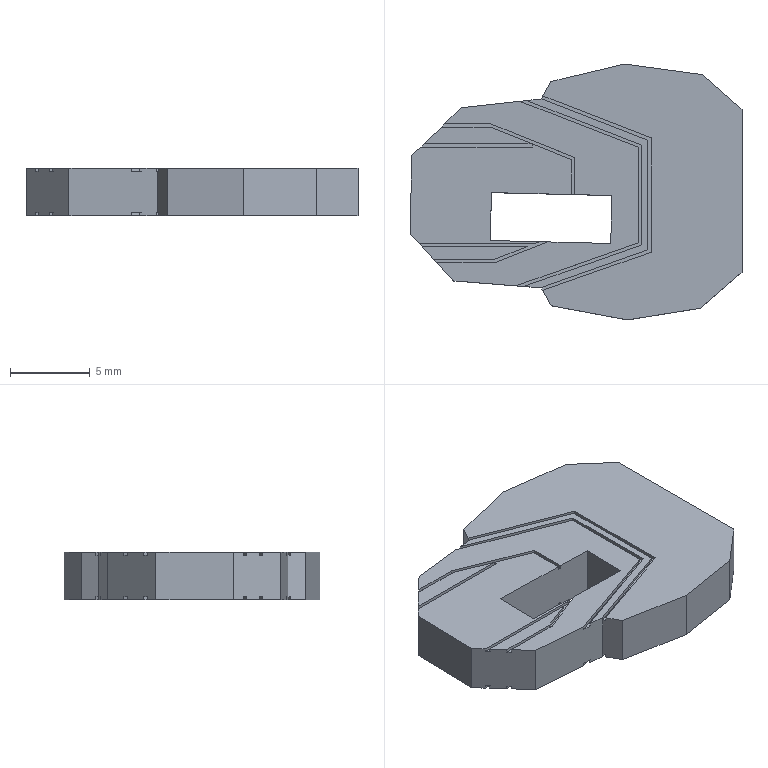Part | SolidWorks | features BaseBody 1 | 1 solid | 96 faces | box 20.777 x 16.014 x 3 mm | volume 719.553 mm3 | plane 84 | spline 12